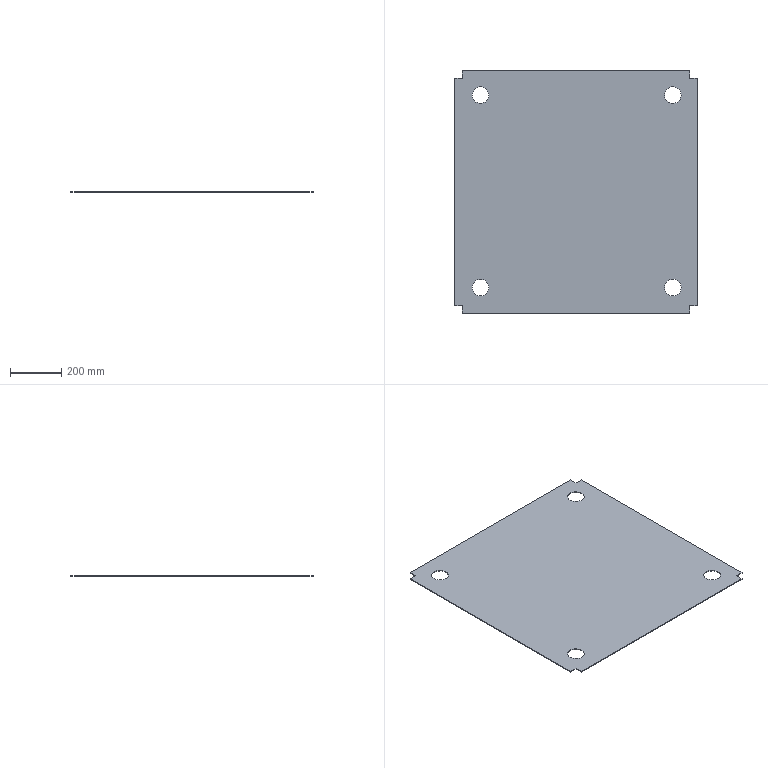Part | STEP file | SynoNew-0304-058 | 1 solid | 18 faces | box 945 x 945 x 3 mm | volume 2628455 mm3 | plane 14 | cylinder 4 | commonest cylinder face diameters 65 x4
STEP:
#1=CARTESIAN_POINT('',(410.,377.5,3.));
#2=VERTEX_POINT('',#1);
#3=CARTESIAN_POINT('',(345.,377.5,3.));
#4=VERTEX_POINT('',#3);
#5=CARTESIAN_POINT('',(377.5,377.5,3.));
#6=DIRECTION('',(0.,0.,-1.));
#7=DIRECTION('',(1.,0.,0.));
#8=AXIS2_PLACEMENT_3D('',#5,#6,#7);
#9=CIRCLE('',#8,32.5);
#10=EDGE_CURVE('',#2,#4,#9,.T.);
#11=ORIENTED_EDGE('',*,*,#10,.F.);
#12=CARTESIAN_POINT('',(377.5,377.5,3.));
#13=DIRECTION('',(0.,0.,-1.));
#14=DIRECTION('',(1.,0.,0.));
#15=AXIS2_PLACEMENT_3D('',#12,#13,#14);
#16=CIRCLE('',#15,32.5);
#17=EDGE_CURVE('',#4,#2,#16,.T.);
#18=ORIENTED_EDGE('',*,*,#17,.F.);
#19=CARTESIAN_POINT('',(345.,377.5,0.));
#20=VERTEX_POINT('',#19);
#21=CARTESIAN_POINT('',(345.,377.5,3.));
#22=DIRECTION('',(0.,0.,-1.));
#23=VECTOR('',#22,32.5);
#24=LINE('',#21,#23);
#25=EDGE_CURVE('',#4,#20,#24,.T.);
#26=ORIENTED_EDGE('',*,*,#25,.T.);
#27=CARTESIAN_POINT('',(410.,377.5,0.));
#28=VERTEX_POINT('',#27);
#29=CARTESIAN_POINT('',(377.5,377.5,0.));
#30=DIRECTION('',(0.,0.,1.));
#31=DIRECTION('',(1.,0.,0.));
#32=AXIS2_PLACEMENT_3D('',#29,#30,#31);
#33=CIRCLE('',#32,32.5);
#34=EDGE_CURVE('',#28,#20,#33,.T.);
#35=ORIENTED_EDGE('',*,*,#34,.F.);
#36=CARTESIAN_POINT('',(377.5,377.5,0.));
#37=DIRECTION('',(0.,0.,1.));
#38=DIRECTION('',(1.,0.,0.));
#39=AXIS2_PLACEMENT_3D('',#36,#37,#38);
#40=CIRCLE('',#39,32.5);
#41=EDGE_CURVE('',#20,#28,#40,.T.);
#42=ORIENTED_EDGE('',*,*,#41,.F.);
#43=ORIENTED_EDGE('',*,*,#25,.F.);
#44=EDGE_LOOP('',(#11,#18,#26,#35,#42,#43));
#45=FACE_OUTER_BOUND('',#44,.T.);
#46=CARTESIAN_POINT('',(377.5,377.5,3.));
#47=DIRECTION('',(0.,0.,-1.));
#48=DIRECTION('',(1.,0.,0.));
#49=AXIS2_PLACEMENT_3D('',#46,#47,#48);
#50=CYLINDRICAL_SURFACE('',#49,32.5);
#51=ADVANCED_FACE('',(#45),#50,.F.);
#52=CARTESIAN_POINT('',(410.,-372.5,3.));
#53=VERTEX_POINT('',#52);
#54=CARTESIAN_POINT('',(345.,-372.5,3.));
#55=VERTEX_POINT('',#54);
#56=CARTESIAN_POINT('',(377.5,-372.5,3.));
#57=DIRECTION('',(0.,0.,-1.));
#58=DIRECTION('',(1.,0.,0.));
#59=AXIS2_PLACEMENT_3D('',#56,#57,#58);
#60=CIRCLE('',#59,32.5);
#61=EDGE_CURVE('',#53,#55,#60,.T.);
#62=ORIENTED_EDGE('',*,*,#61,.F.);
#63=CARTESIAN_POINT('',(377.5,-372.5,3.));
#64=DIRECTION('',(0.,0.,-1.));
#65=DIRECTION('',(1.,0.,0.));
#66=AXIS2_PLACEMENT_3D('',#63,#64,#65);
#67=CIRCLE('',#66,32.5);
#68=EDGE_CURVE('',#55,#53,#67,.T.);
#69=ORIENTED_EDGE('',*,*,#68,.F.);
#70=CARTESIAN_POINT('',(345.,-372.5,0.));
#71=VERTEX_POINT('',#70);
#72=CARTESIAN_POINT('',(345.,-372.5,3.));
#73=DIRECTION('',(0.,0.,-1.));
#74=VECTOR('',#73,32.5);
#75=LINE('',#72,#74);
#76=EDGE_CURVE('',#55,#71,#75,.T.);
#77=ORIENTED_EDGE('',*,*,#76,.T.);
#78=CARTESIAN_POINT('',(410.,-372.5,0.));
#79=VERTEX_POINT('',#78);
#80=CARTESIAN_POINT('',(377.5,-372.5,0.));
#81=DIRECTION('',(0.,0.,1.));
#82=DIRECTION('',(1.,0.,0.));
#83=AXIS2_PLACEMENT_3D('',#80,#81,#82);
#84=CIRCLE('',#83,32.5);
#85=EDGE_CURVE('',#79,#71,#84,.T.);
#86=ORIENTED_EDGE('',*,*,#85,.F.);
#87=CARTESIAN_POINT('',(377.5,-372.5,0.));
#88=DIRECTION('',(0.,0.,1.));
#89=DIRECTION('',(1.,0.,0.));
#90=AXIS2_PLACEMENT_3D('',#87,#88,#89);
#91=CIRCLE('',#90,32.5);
#92=EDGE_CURVE('',#71,#79,#91,.T.);
#93=ORIENTED_EDGE('',*,*,#92,.F.);
#94=ORIENTED_EDGE('',*,*,#76,.F.);
#95=EDGE_LOOP('',(#62,#69,#77,#86,#93,#94));
#96=FACE_OUTER_BOUND('',#95,.T.);
#97=CARTESIAN_POINT('',(377.5,-372.5,3.));
#98=DIRECTION('',(0.,0.,-1.));
#99=DIRECTION('',(1.,0.,0.));
#100=AXIS2_PLACEMENT_3D('',#97,#98,#99);
#101=CYLINDRICAL_SURFACE('',#100,32.5);
#102=ADVANCED_FACE('',(#96),#101,.F.);
#103=CARTESIAN_POINT('',(-340.,377.5,3.));
#104=VERTEX_POINT('',#103);
#105=CARTESIAN_POINT('',(-405.,377.5,3.));
#106=VERTEX_POINT('',#105);
#107=CARTESIAN_POINT('',(-372.5,377.5,3.));
#108=DIRECTION('',(0.,0.,-1.));
#109=DIRECTION('',(1.,0.,0.));
#110=AXIS2_PLACEMENT_3D('',#107,#108,#109);
#111=CIRCLE('',#110,32.5);
#112=EDGE_CURVE('',#104,#106,#111,.T.);
#113=ORIENTED_EDGE('',*,*,#112,.F.);
#114=CARTESIAN_POINT('',(-372.5,377.5,3.));
#115=DIRECTION('',(0.,0.,-1.));
#116=DIRECTION('',(1.,0.,0.));
#117=AXIS2_PLACEMENT_3D('',#114,#115,#116);
#118=CIRCLE('',#117,32.5);
#119=EDGE_CURVE('',#106,#104,#118,.T.);
#120=ORIENTED_EDGE('',*,*,#119,.F.);
#121=CARTESIAN_POINT('',(-405.,377.5,0.));
#122=VERTEX_POINT('',#121);
#123=CARTESIAN_POINT('',(-405.,377.5,3.));
#124=DIRECTION('',(0.,0.,-1.));
#125=VECTOR('',#124,32.5);
#126=LINE('',#123,#125);
#127=EDGE_CURVE('',#106,#122,#126,.T.);
#128=ORIENTED_EDGE('',*,*,#127,.T.);
#129=CARTESIAN_POINT('',(-340.,377.5,0.));
#130=VERTEX_POINT('',#129);
#131=CARTESIAN_POINT('',(-372.5,377.5,0.));
#132=DIRECTION('',(0.,0.,1.));
#133=DIRECTION('',(1.,0.,0.));
#134=AXIS2_PLACEMENT_3D('',#131,#132,#133);
#135=CIRCLE('',#134,32.5);
#136=EDGE_CURVE('',#130,#122,#135,.T.);
#137=ORIENTED_EDGE('',*,*,#136,.F.);
#138=CARTESIAN_POINT('',(-372.5,377.5,0.));
#139=DIRECTION('',(0.,0.,1.));
#140=DIRECTION('',(1.,0.,0.));
#141=AXIS2_PLACEMENT_3D('',#138,#139,#140);
#142=CIRCLE('',#141,32.5);
#143=EDGE_CURVE('',#122,#130,#142,.T.);
#144=ORIENTED_EDGE('',*,*,#143,.F.);
#145=ORIENTED_EDGE('',*,*,#127,.F.);
#146=EDGE_LOOP('',(#113,#120,#128,#137,#144,#145));
#147=FACE_OUTER_BOUND('',#146,.T.);
#148=CARTESIAN_POINT('',(-372.5,377.5,3.));
#149=DIRECTION('',(0.,0.,-1.));
#150=DIRECTION('',(1.,0.,0.));
#151=AXIS2_PLACEMENT_3D('',#148,#149,#150);
#152=CYLINDRICAL_SURFACE('',#151,32.5);
#153=ADVANCED_FACE('',(#147),#152,.F.);
#154=CARTESIAN_POINT('',(-340.,-372.5,3.));
#155=VERTEX_POINT('',#154);
#156=CARTESIAN_POINT('',(-405.,-372.5,3.));
#157=VERTEX_POINT('',#156);
#158=CARTESIAN_POINT('',(-372.5,-372.5,3.));
#159=DIRECTION('',(0.,0.,-1.));
#160=DIRECTION('',(1.,0.,0.));
#161=AXIS2_PLACEMENT_3D('',#158,#159,#160);
#162=CIRCLE('',#161,32.5);
#163=EDGE_CURVE('',#155,#157,#162,.T.);
#164=ORIENTED_EDGE('',*,*,#163,.F.);
#165=CARTESIAN_POINT('',(-372.5,-372.5,3.));
#166=DIRECTION('',(0.,0.,-1.));
#167=DIRECTION('',(1.,0.,0.));
#168=AXIS2_PLACEMENT_3D('',#165,#166,#167);
#169=CIRCLE('',#168,32.5);
#170=EDGE_CURVE('',#157,#155,#169,.T.);
#171=ORIENTED_EDGE('',*,*,#170,.F.);
#172=CARTESIAN_POINT('',(-405.,-372.5,0.));
#173=VERTEX_POINT('',#172);
#174=CARTESIAN_POINT('',(-405.,-372.5,3.));
#175=DIRECTION('',(0.,0.,-1.));
#176=VECTOR('',#175,32.5);
#177=LINE('',#174,#176);
#178=EDGE_CURVE('',#157,#173,#177,.T.);
#179=ORIENTED_EDGE('',*,*,#178,.T.);
#180=CARTESIAN_POINT('',(-340.,-372.5,0.));
#181=VERTEX_POINT('',#180);
#182=CARTESIAN_POINT('',(-372.5,-372.5,0.));
#183=DIRECTION('',(0.,0.,1.));
#184=DIRECTION('',(1.,0.,0.));
#185=AXIS2_PLACEMENT_3D('',#182,#183,#184);
#186=CIRCLE('',#185,32.5);
#187=EDGE_CURVE('',#181,#173,#186,.T.);
#188=ORIENTED_EDGE('',*,*,#187,.F.);
#189=CARTESIAN_POINT('',(-372.5,-372.5,0.));
#190=DIRECTION('',(0.,0.,1.));
#191=DIRECTION('',(1.,0.,0.));
#192=AXIS2_PLACEMENT_3D('',#189,#190,#191);
#193=CIRCLE('',#192,32.5);
#194=EDGE_CURVE('',#173,#181,#193,.T.);
#195=ORIENTED_EDGE('',*,*,#194,.F.);
#196=ORIENTED_EDGE('',*,*,#178,.F.);
#197=EDGE_LOOP('',(#164,#171,#179,#188,#195,#196));
#198=FACE_OUTER_BOUND('',#197,.T.);
#199=CARTESIAN_POINT('',(-372.5,-372.5,3.));
#200=DIRECTION('',(0.,0.,-1.));
#201=DIRECTION('',(1.,0.,0.));
#202=AXIS2_PLACEMENT_3D('',#199,#200,#201);
#203=CYLINDRICAL_SURFACE('',#202,32.5);
#204=ADVANCED_FACE('',(#198),#203,.F.);
#205=CARTESIAN_POINT('',(472.5,-442.5,3.));
#206=VERTEX_POINT('',#205);
#207=CARTESIAN_POINT('',(472.5,-442.5,0.));
#208=VERTEX_POINT('',#207);
#209=CARTESIAN_POINT('',(472.5,-442.5,1.5));
#210=DIRECTION('',(0.,0.,-1.));
#211=VECTOR('',#210,10.);
#212=LINE('',#209,#211);
#213=EDGE_CURVE('',#206,#208,#212,.T.);
#214=ORIENTED_EDGE('',*,*,#213,.F.);
#215=CARTESIAN_POINT('',(442.5,-442.5,3.));
#216=VERTEX_POINT('',#215);
#217=CARTESIAN_POINT('',(247.537,-442.5,3.));
#218=DIRECTION('',(1.,0.,0.));
#219=VECTOR('',#218,10.);
#220=LINE('',#217,#219);
#221=EDGE_CURVE('',#216,#206,#220,.T.);
#222=ORIENTED_EDGE('',*,*,#221,.F.);
#223=CARTESIAN_POINT('',(442.5,-442.5,0.));
#224=VERTEX_POINT('',#223);
#225=CARTESIAN_POINT('',(442.5,-442.5,3.));
#226=DIRECTION('',(0.,0.,-1.));
#227=VECTOR('',#226,10.);
#228=LINE('',#225,#227);
#229=EDGE_CURVE('',#216,#224,#228,.T.);
#230=ORIENTED_EDGE('',*,*,#229,.T.);
#231=CARTESIAN_POINT('',(247.537,-442.5,0.));
#232=DIRECTION('',(-1.,0.,0.));
#233=VECTOR('',#232,10.);
#234=LINE('',#231,#233);
#235=EDGE_CURVE('',#208,#224,#234,.T.);
#236=ORIENTED_EDGE('',*,*,#235,.F.);
#237=EDGE_LOOP('',(#214,#222,#230,#236));
#238=FACE_OUTER_BOUND('',#237,.T.);
#239=CARTESIAN_POINT('',(495.074,-442.5,3.));
#240=DIRECTION('',(0.,-1.,0.));
#241=DIRECTION('',(-1.,0.,0.));
#242=AXIS2_PLACEMENT_3D('',#239,#240,#241);
#243=PLANE('',#242);
#244=ADVANCED_FACE('',(#238),#243,.T.);
#245=CARTESIAN_POINT('',(442.5,-472.5,0.));
#246=VERTEX_POINT('',#245);
#247=CARTESIAN_POINT('',(442.5,-221.25,0.));
#248=DIRECTION('',(0.,-1.,0.));
#249=VECTOR('',#248,10.);
#250=LINE('',#247,#249);
#251=EDGE_CURVE('',#224,#246,#250,.T.);
#252=ORIENTED_EDGE('',*,*,#251,.F.);
#253=ORIENTED_EDGE('',*,*,#229,.F.);
#254=CARTESIAN_POINT('',(442.5,-472.5,3.));
#255=VERTEX_POINT('',#254);
#256=CARTESIAN_POINT('',(442.5,-221.25,3.));
#257=DIRECTION('',(0.,1.,0.));
#258=VECTOR('',#257,10.);
#259=LINE('',#256,#258);
#260=EDGE_CURVE('',#255,#216,#259,.T.);
#261=ORIENTED_EDGE('',*,*,#260,.F.);
#262=CARTESIAN_POINT('',(442.5,-472.5,1.5));
#263=DIRECTION('',(0.,0.,1.));
#264=VECTOR('',#263,10.);
#265=LINE('',#262,#264);
#266=EDGE_CURVE('',#246,#255,#265,.T.);
#267=ORIENTED_EDGE('',*,*,#266,.F.);
#268=EDGE_LOOP('',(#252,#253,#261,#267));
#269=FACE_OUTER_BOUND('',#268,.T.);
#270=CARTESIAN_POINT('',(442.5,-442.5,3.));
#271=DIRECTION('',(1.,0.,0.));
#272=DIRECTION('',(0.,-1.,0.));
#273=AXIS2_PLACEMENT_3D('',#270,#271,#272);
#274=PLANE('',#273);
#275=ADVANCED_FACE('',(#269),#274,.T.);
#276=CARTESIAN_POINT('',(-442.5,-472.5,0.));
#277=VERTEX_POINT('',#276);
#278=CARTESIAN_POINT('',(-442.5,-442.5,0.));
#279=VERTEX_POINT('',#278);
#280=CARTESIAN_POINT('',(-442.5,-244.911,0.));
#281=DIRECTION('',(0.,1.,0.));
#282=VECTOR('',#281,10.);
#283=LINE('',#280,#282);
#284=EDGE_CURVE('',#277,#279,#283,.T.);
#285=ORIENTED_EDGE('',*,*,#284,.F.);
#286=CARTESIAN_POINT('',(-442.5,-472.5,3.));
#287=VERTEX_POINT('',#286);
#288=CARTESIAN_POINT('',(-442.5,-472.5,1.5));
#289=DIRECTION('',(0.,0.,-1.));
#290=VECTOR('',#289,10.);
#291=LINE('',#288,#290);
#292=EDGE_CURVE('',#287,#277,#291,.T.);
#293=ORIENTED_EDGE('',*,*,#292,.F.);
#294=CARTESIAN_POINT('',(-442.5,-442.5,3.));
#295=VERTEX_POINT('',#294);
#296=CARTESIAN_POINT('',(-442.5,-244.911,3.));
#297=DIRECTION('',(0.,-1.,0.));
#298=VECTOR('',#297,10.);
#299=LINE('',#296,#298);
#300=EDGE_CURVE('',#295,#287,#299,.T.);
#301=ORIENTED_EDGE('',*,*,#300,.F.);
#302=CARTESIAN_POINT('',(-442.5,-442.5,3.));
#303=DIRECTION('',(0.,0.,-1.));
#304=VECTOR('',#303,10.);
#305=LINE('',#302,#304);
#306=EDGE_CURVE('',#295,#279,#305,.T.);
#307=ORIENTED_EDGE('',*,*,#306,.T.);
#308=EDGE_LOOP('',(#285,#293,#301,#307));
#309=FACE_OUTER_BOUND('',#308,.T.);
#310=CARTESIAN_POINT('',(-442.5,-489.822,3.));
#311=DIRECTION('',(-1.,0.,0.));
#312=DIRECTION('',(0.,1.,0.));
#313=AXIS2_PLACEMENT_3D('',#310,#311,#312);
#314=PLANE('',#313);
#315=ADVANCED_FACE('',(#309),#314,.T.);
#316=CARTESIAN_POINT('',(-472.5,-442.5,0.));
#317=VERTEX_POINT('',#316);
#318=CARTESIAN_POINT('',(-472.5,-442.5,3.));
#319=VERTEX_POINT('',#318);
#320=CARTESIAN_POINT('',(-472.5,-442.5,1.5));
#321=DIRECTION('',(0.,0.,1.));
#322=VECTOR('',#321,10.);
#323=LINE('',#320,#322);
#324=EDGE_CURVE('',#317,#319,#323,.T.);
#325=ORIENTED_EDGE('',*,*,#324,.F.);
#326=CARTESIAN_POINT('',(-221.25,-442.5,0.));
#327=DIRECTION('',(-1.,0.,0.));
#328=VECTOR('',#327,10.);
#329=LINE('',#326,#328);
#330=EDGE_CURVE('',#279,#317,#329,.T.);
#331=ORIENTED_EDGE('',*,*,#330,.F.);
#332=ORIENTED_EDGE('',*,*,#306,.F.);
#333=CARTESIAN_POINT('',(-221.25,-442.5,3.));
#334=DIRECTION('',(1.,0.,0.));
#335=VECTOR('',#334,10.);
#336=LINE('',#333,#335);
#337=EDGE_CURVE('',#319,#295,#336,.T.);
#338=ORIENTED_EDGE('',*,*,#337,.F.);
#339=EDGE_LOOP('',(#325,#331,#332,#338));
#340=FACE_OUTER_BOUND('',#339,.T.);
#341=CARTESIAN_POINT('',(-442.5,-442.5,3.));
#342=DIRECTION('',(0.,-1.,0.));
#343=DIRECTION('',(-1.,0.,0.));
#344=AXIS2_PLACEMENT_3D('',#341,#342,#343);
#345=PLANE('',#344);
#346=ADVANCED_FACE('',(#340),#345,.T.);
#347=ORIENTED_EDGE('',*,*,#266,.T.);
#348=CARTESIAN_POINT('',(-472.5,-472.5,3.));
#349=DIRECTION('',(1.,0.,0.));
#350=VECTOR('',#349,10.);
#351=LINE('',#348,#350);
#352=EDGE_CURVE('',#287,#255,#351,.T.);
#353=ORIENTED_EDGE('',*,*,#352,.F.);
#354=ORIENTED_EDGE('',*,*,#292,.T.);
#355=CARTESIAN_POINT('',(-472.5,-472.5,0.));
#356=DIRECTION('',(1.,0.,0.));
#357=VECTOR('',#356,10.);
#358=LINE('',#355,#357);
#359=EDGE_CURVE('',#277,#246,#358,.T.);
#360=ORIENTED_EDGE('',*,*,#359,.T.);
#361=EDGE_LOOP('',(#347,#353,#354,#360));
#362=FACE_OUTER_BOUND('',#361,.T.);
#363=CARTESIAN_POINT('',(-472.5,-472.5,0.));
#364=DIRECTION('',(0.,-1.,0.));
#365=DIRECTION('',(1.,0.,0.));
#366=AXIS2_PLACEMENT_3D('',#363,#364,#365);
#367=PLANE('',#366);
#368=ADVANCED_FACE('',(#362),#367,.T.);
#369=ORIENTED_EDGE('',*,*,#260,.T.);
#370=ORIENTED_EDGE('',*,*,#221,.T.);
#371=CARTESIAN_POINT('',(472.5,442.5,3.));
#372=VERTEX_POINT('',#371);
#373=CARTESIAN_POINT('',(472.5,-472.5,3.));
#374=DIRECTION('',(0.,1.,0.));
#375=VECTOR('',#374,10.);
#376=LINE('',#373,#375);
#377=EDGE_CURVE('',#206,#372,#376,.T.);
#378=ORIENTED_EDGE('',*,*,#377,.T.);
#379=CARTESIAN_POINT('',(442.5,442.5,3.));
#380=VERTEX_POINT('',#379);
#381=CARTESIAN_POINT('',(247.537,442.5,3.));
#382=DIRECTION('',(-1.,0.,0.));
#383=VECTOR('',#382,10.);
#384=LINE('',#381,#383);
#385=EDGE_CURVE('',#372,#380,#384,.T.);
#386=ORIENTED_EDGE('',*,*,#385,.T.);
#387=CARTESIAN_POINT('',(442.5,472.5,3.));
#388=VERTEX_POINT('',#387);
#389=CARTESIAN_POINT('',(442.5,221.25,3.));
#390=DIRECTION('',(0.,1.,0.));
#391=VECTOR('',#390,10.);
#392=LINE('',#389,#391);
#393=EDGE_CURVE('',#380,#388,#392,.T.);
#394=ORIENTED_EDGE('',*,*,#393,.T.);
#395=CARTESIAN_POINT('',(-442.5,472.5,3.));
#396=VERTEX_POINT('',#395);
#397=CARTESIAN_POINT('',(472.5,472.5,3.));
#398=DIRECTION('',(-1.,0.,0.));
#399=VECTOR('',#398,10.);
#400=LINE('',#397,#399);
#401=EDGE_CURVE('',#388,#396,#400,.T.);
#402=ORIENTED_EDGE('',*,*,#401,.T.);
#403=CARTESIAN_POINT('',(-442.5,442.5,3.));
#404=VERTEX_POINT('',#403);
#405=CARTESIAN_POINT('',(-442.5,244.911,3.));
#406=DIRECTION('',(0.,-1.,0.));
#407=VECTOR('',#406,10.);
#408=LINE('',#405,#407);
#409=EDGE_CURVE('',#396,#404,#408,.T.);
#410=ORIENTED_EDGE('',*,*,#409,.T.);
#411=CARTESIAN_POINT('',(-472.5,442.5,3.));
#412=VERTEX_POINT('',#411);
#413=CARTESIAN_POINT('',(-221.25,442.5,3.));
#414=DIRECTION('',(-1.,0.,0.));
#415=VECTOR('',#414,10.);
#416=LINE('',#413,#415);
#417=EDGE_CURVE('',#404,#412,#416,.T.);
#418=ORIENTED_EDGE('',*,*,#417,.T.);
#419=CARTESIAN_POINT('',(-472.5,472.5,3.));
#420=DIRECTION('',(0.,-1.,0.));
#421=VECTOR('',#420,10.);
#422=LINE('',#419,#421);
#423=EDGE_CURVE('',#412,#319,#422,.T.);
#424=ORIENTED_EDGE('',*,*,#423,.T.);
#425=ORIENTED_EDGE('',*,*,#337,.T.);
#426=ORIENTED_EDGE('',*,*,#300,.T.);
#427=ORIENTED_EDGE('',*,*,#352,.T.);
#428=EDGE_LOOP('',(#369,#370,#378,#386,#394,#402,#410,#418,#424,#425,#426,#427));
#429=FACE_OUTER_BOUND('',#428,.T.);
#430=ORIENTED_EDGE('',*,*,#10,.T.);
#431=ORIENTED_EDGE('',*,*,#17,.T.);
#432=EDGE_LOOP('',(#430,#431));
#433=FACE_BOUND('',#432,.T.);
#434=ORIENTED_EDGE('',*,*,#61,.T.);
#435=ORIENTED_EDGE('',*,*,#68,.T.);
#436=EDGE_LOOP('',(#434,#435));
#437=FACE_BOUND('',#436,.T.);
#438=ORIENTED_EDGE('',*,*,#112,.T.);
#439=ORIENTED_EDGE('',*,*,#119,.T.);
#440=EDGE_LOOP('',(#438,#439));
#441=FACE_BOUND('',#440,.T.);
#442=ORIENTED_EDGE('',*,*,#163,.T.);
#443=ORIENTED_EDGE('',*,*,#170,.T.);
#444=EDGE_LOOP('',(#442,#443));
#445=FACE_BOUND('',#444,.T.);
#446=CARTESIAN_POINT('',(0.,0.,3.));
#447=DIRECTION('',(0.,0.,1.));
#448=DIRECTION('',(1.,0.,0.));
#449=AXIS2_PLACEMENT_3D('',#446,#447,#448);
#450=PLANE('',#449);
#451=ADVANCED_FACE('',(#429,#433,#437,#441,#445),#450,.T.);
#452=ORIENTED_EDGE('',*,*,#324,.T.);
#453=ORIENTED_EDGE('',*,*,#423,.F.);
#454=CARTESIAN_POINT('',(-472.5,442.5,0.));
#455=VERTEX_POINT('',#454);
#456=CARTESIAN_POINT('',(-472.5,442.5,1.5));
#457=DIRECTION('',(0.,0.,-1.));
#458=VECTOR('',#457,10.);
#459=LINE('',#456,#458);
#460=EDGE_CURVE('',#412,#455,#459,.T.);
#461=ORIENTED_EDGE('',*,*,#460,.T.);
#462=CARTESIAN_POINT('',(-472.5,472.5,0.));
#463=DIRECTION('',(0.,-1.,0.));
#464=VECTOR('',#463,10.);
#465=LINE('',#462,#464);
#466=EDGE_CURVE('',#455,#317,#465,.T.);
#467=ORIENTED_EDGE('',*,*,#466,.T.);
#468=EDGE_LOOP('',(#452,#453,#461,#467));
#469=FACE_OUTER_BOUND('',#468,.T.);
#470=CARTESIAN_POINT('',(-472.5,472.5,0.));
#471=DIRECTION('',(-1.,0.,0.));
#472=DIRECTION('',(0.,-1.,0.));
#473=AXIS2_PLACEMENT_3D('',#470,#471,#472);
#474=PLANE('',#473);
#475=ADVANCED_FACE('',(#469),#474,.T.);
#476=CARTESIAN_POINT('',(472.5,442.5,0.));
#477=VERTEX_POINT('',#476);
#478=CARTESIAN_POINT('',(472.5,442.5,1.5));
#479=DIRECTION('',(0.,0.,1.));
#480=VECTOR('',#479,10.);
#481=LINE('',#478,#480);
#482=EDGE_CURVE('',#477,#372,#481,.T.);
#483=ORIENTED_EDGE('',*,*,#482,.F.);
#484=CARTESIAN_POINT('',(442.5,442.5,0.));
#485=VERTEX_POINT('',#484);
#486=CARTESIAN_POINT('',(247.537,442.5,0.));
#487=DIRECTION('',(1.,0.,0.));
#488=VECTOR('',#487,10.);
#489=LINE('',#486,#488);
#490=EDGE_CURVE('',#485,#477,#489,.T.);
#491=ORIENTED_EDGE('',*,*,#490,.F.);
#492=CARTESIAN_POINT('',(442.5,442.5,3.));
#493=DIRECTION('',(0.,0.,-1.));
#494=VECTOR('',#493,10.);
#495=LINE('',#492,#494);
#496=EDGE_CURVE('',#380,#485,#495,.T.);
#497=ORIENTED_EDGE('',*,*,#496,.F.);
#498=ORIENTED_EDGE('',*,*,#385,.F.);
#499=EDGE_LOOP('',(#483,#491,#497,#498));
#500=FACE_OUTER_BOUND('',#499,.T.);
#501=CARTESIAN_POINT('',(495.074,442.5,3.));
#502=DIRECTION('',(0.,-1.,0.));
#503=DIRECTION('',(-1.,0.,0.));
#504=AXIS2_PLACEMENT_3D('',#501,#502,#503);
#505=PLANE('',#504);
#506=ADVANCED_FACE('',(#500),#505,.F.);
#507=CARTESIAN_POINT('',(442.5,472.5,0.));
#508=VERTEX_POINT('',#507);
#509=CARTESIAN_POINT('',(442.5,221.25,0.));
#510=DIRECTION('',(0.,-1.,0.));
#511=VECTOR('',#510,10.);
#512=LINE('',#509,#511);
#513=EDGE_CURVE('',#508,#485,#512,.T.);
#514=ORIENTED_EDGE('',*,*,#513,.F.);
#515=CARTESIAN_POINT('',(442.5,472.5,1.5));
#516=DIRECTION('',(0.,0.,-1.));
#517=VECTOR('',#516,10.);
#518=LINE('',#515,#517);
#519=EDGE_CURVE('',#388,#508,#518,.T.);
#520=ORIENTED_EDGE('',*,*,#519,.F.);
#521=ORIENTED_EDGE('',*,*,#393,.F.);
#522=ORIENTED_EDGE('',*,*,#496,.T.);
#523=EDGE_LOOP('',(#514,#520,#521,#522));
#524=FACE_OUTER_BOUND('',#523,.T.);
#525=CARTESIAN_POINT('',(442.5,442.5,3.));
#526=DIRECTION('',(-1.,0.,0.));
#527=DIRECTION('',(0.,1.,0.));
#528=AXIS2_PLACEMENT_3D('',#525,#526,#527);
#529=PLANE('',#528);
#530=ADVANCED_FACE('',(#524),#529,.F.);
#531=ORIENTED_EDGE('',*,*,#460,.F.);
#532=ORIENTED_EDGE('',*,*,#417,.F.);
#533=CARTESIAN_POINT('',(-442.5,442.5,0.));
#534=VERTEX_POINT('',#533);
#535=CARTESIAN_POINT('',(-442.5,442.5,3.));
#536=DIRECTION('',(0.,0.,-1.));
#537=VECTOR('',#536,10.);
#538=LINE('',#535,#537);
#539=EDGE_CURVE('',#404,#534,#538,.T.);
#540=ORIENTED_EDGE('',*,*,#539,.T.);
#541=CARTESIAN_POINT('',(-221.25,442.5,0.));
#542=DIRECTION('',(1.,0.,0.));
#543=VECTOR('',#542,10.);
#544=LINE('',#541,#543);
#545=EDGE_CURVE('',#455,#534,#544,.T.);
#546=ORIENTED_EDGE('',*,*,#545,.F.);
#547=EDGE_LOOP('',(#531,#532,#540,#546));
#548=FACE_OUTER_BOUND('',#547,.T.);
#549=CARTESIAN_POINT('',(-442.5,442.5,3.));
#550=DIRECTION('',(0.,-1.,0.));
#551=DIRECTION('',(-1.,0.,0.));
#552=AXIS2_PLACEMENT_3D('',#549,#550,#551);
#553=PLANE('',#552);
#554=ADVANCED_FACE('',(#548),#553,.F.);
#555=CARTESIAN_POINT('',(-442.5,472.5,0.));
#556=VERTEX_POINT('',#555);
#557=CARTESIAN_POINT('',(-442.5,244.911,0.));
#558=DIRECTION('',(0.,1.,0.));
#559=VECTOR('',#558,10.);
#560=LINE('',#557,#559);
#561=EDGE_CURVE('',#534,#556,#560,.T.);
#562=ORIENTED_EDGE('',*,*,#561,.F.);
#563=ORIENTED_EDGE('',*,*,#539,.F.);
#564=ORIENTED_EDGE('',*,*,#409,.F.);
#565=CARTESIAN_POINT('',(-442.5,472.5,1.5));
#566=DIRECTION('',(0.,0.,1.));
#567=VECTOR('',#566,10.);
#568=LINE('',#565,#567);
#569=EDGE_CURVE('',#556,#396,#568,.T.);
#570=ORIENTED_EDGE('',*,*,#569,.F.);
#571=EDGE_LOOP('',(#562,#563,#564,#570));
#572=FACE_OUTER_BOUND('',#571,.T.);
#573=CARTESIAN_POINT('',(-442.5,489.822,3.));
#574=DIRECTION('',(1.,0.,0.));
#575=DIRECTION('',(0.,-1.,0.));
#576=AXIS2_PLACEMENT_3D('',#573,#574,#575);
#577=PLANE('',#576);
#578=ADVANCED_FACE('',(#572),#577,.F.);
#579=ORIENTED_EDGE('',*,*,#213,.T.);
#580=CARTESIAN_POINT('',(472.5,-472.5,0.));
#581=DIRECTION('',(0.,1.,0.));
#582=VECTOR('',#581,10.);
#583=LINE('',#580,#582);
#584=EDGE_CURVE('',#208,#477,#583,.T.);
#585=ORIENTED_EDGE('',*,*,#584,.T.);
#586=ORIENTED_EDGE('',*,*,#482,.T.);
#587=ORIENTED_EDGE('',*,*,#377,.F.);
#588=EDGE_LOOP('',(#579,#585,#586,#587));
#589=FACE_OUTER_BOUND('',#588,.T.);
#590=CARTESIAN_POINT('',(472.5,-472.5,0.));
#591=DIRECTION('',(1.,0.,0.));
#592=DIRECTION('',(0.,1.,0.));
#593=AXIS2_PLACEMENT_3D('',#590,#591,#592);
#594=PLANE('',#593);
#595=ADVANCED_FACE('',(#589),#594,.T.);
#596=ORIENTED_EDGE('',*,*,#519,.T.);
#597=CARTESIAN_POINT('',(472.5,472.5,0.));
#598=DIRECTION('',(-1.,0.,0.));
#599=VECTOR('',#598,10.);
#600=LINE('',#597,#599);
#601=EDGE_CURVE('',#508,#556,#600,.T.);
#602=ORIENTED_EDGE('',*,*,#601,.T.);
#603=ORIENTED_EDGE('',*,*,#569,.T.);
#604=ORIENTED_EDGE('',*,*,#401,.F.);
#605=EDGE_LOOP('',(#596,#602,#603,#604));
#606=FACE_OUTER_BOUND('',#605,.T.);
#607=CARTESIAN_POINT('',(472.5,472.5,0.));
#608=DIRECTION('',(0.,1.,0.));
#609=DIRECTION('',(-1.,0.,0.));
#610=AXIS2_PLACEMENT_3D('',#607,#608,#609);
#611=PLANE('',#610);
#612=ADVANCED_FACE('',(#606),#611,.T.);
#613=ORIENTED_EDGE('',*,*,#251,.T.);
#614=ORIENTED_EDGE('',*,*,#359,.F.);
#615=ORIENTED_EDGE('',*,*,#284,.T.);
#616=ORIENTED_EDGE('',*,*,#330,.T.);
#617=ORIENTED_EDGE('',*,*,#466,.F.);
#618=ORIENTED_EDGE('',*,*,#545,.T.);
#619=ORIENTED_EDGE('',*,*,#561,.T.);
#620=ORIENTED_EDGE('',*,*,#601,.F.);
#621=ORIENTED_EDGE('',*,*,#513,.T.);
#622=ORIENTED_EDGE('',*,*,#490,.T.);
#623=ORIENTED_EDGE('',*,*,#584,.F.);
#624=ORIENTED_EDGE('',*,*,#235,.T.);
#625=EDGE_LOOP('',(#613,#614,#615,#616,#617,#618,#619,#620,#621,#622,#623,#624));
#626=FACE_OUTER_BOUND('',#625,.T.);
#627=ORIENTED_EDGE('',*,*,#34,.T.);
#628=ORIENTED_EDGE('',*,*,#41,.T.);
#629=EDGE_LOOP('',(#627,#628));
#630=FACE_BOUND('',#629,.T.);
#631=ORIENTED_EDGE('',*,*,#85,.T.);
#632=ORIENTED_EDGE('',*,*,#92,.T.);
#633=EDGE_LOOP('',(#631,#632));
#634=FACE_BOUND('',#633,.T.);
#635=ORIENTED_EDGE('',*,*,#136,.T.);
#636=ORIENTED_EDGE('',*,*,#143,.T.);
#637=EDGE_LOOP('',(#635,#636));
#638=FACE_BOUND('',#637,.T.);
#639=ORIENTED_EDGE('',*,*,#187,.T.);
#640=ORIENTED_EDGE('',*,*,#194,.T.);
#641=EDGE_LOOP('',(#639,#640));
#642=FACE_BOUND('',#641,.T.);
#643=CARTESIAN_POINT('',(0.,0.,0.));
#644=DIRECTION('',(0.,0.,1.));
#645=DIRECTION('',(1.,0.,0.));
#646=AXIS2_PLACEMENT_3D('',#643,#644,#645);
#647=PLANE('',#646);
#648=ADVANCED_FACE('',(#626,#630,#634,#638,#642),#647,.F.);
#649=CLOSED_SHELL('',(#51,#102,#153,#204,#244,#275,#315,#346,#368,#451,#475,#506,#530,#554,#578,#595,#612,#648));
#650=MANIFOLD_SOLID_BREP('',#649);
#651=(LENGTH_UNIT()NAMED_UNIT(*)SI_UNIT(.MILLI.,.METRE.));
#652=UNCERTAINTY_MEASURE_WITH_UNIT(LENGTH_MEASURE(0.01),#651,'','');
#653=(NAMED_UNIT(*)PLANE_ANGLE_UNIT()SI_UNIT($,.RADIAN.));
#654=(NAMED_UNIT(*)SI_UNIT($,.STERADIAN.)SOLID_ANGLE_UNIT());
#655=(GEOMETRIC_REPRESENTATION_CONTEXT(3)GLOBAL_UNCERTAINTY_ASSIGNED_CONTEXT((#652))GLOBAL_UNIT_ASSIGNED_CONTEXT((#651,#653,#654))REPRESENTATION_CONTEXT('',''));
#656=ADVANCED_BREP_SHAPE_REPRESENTATION('',(#650),#655);